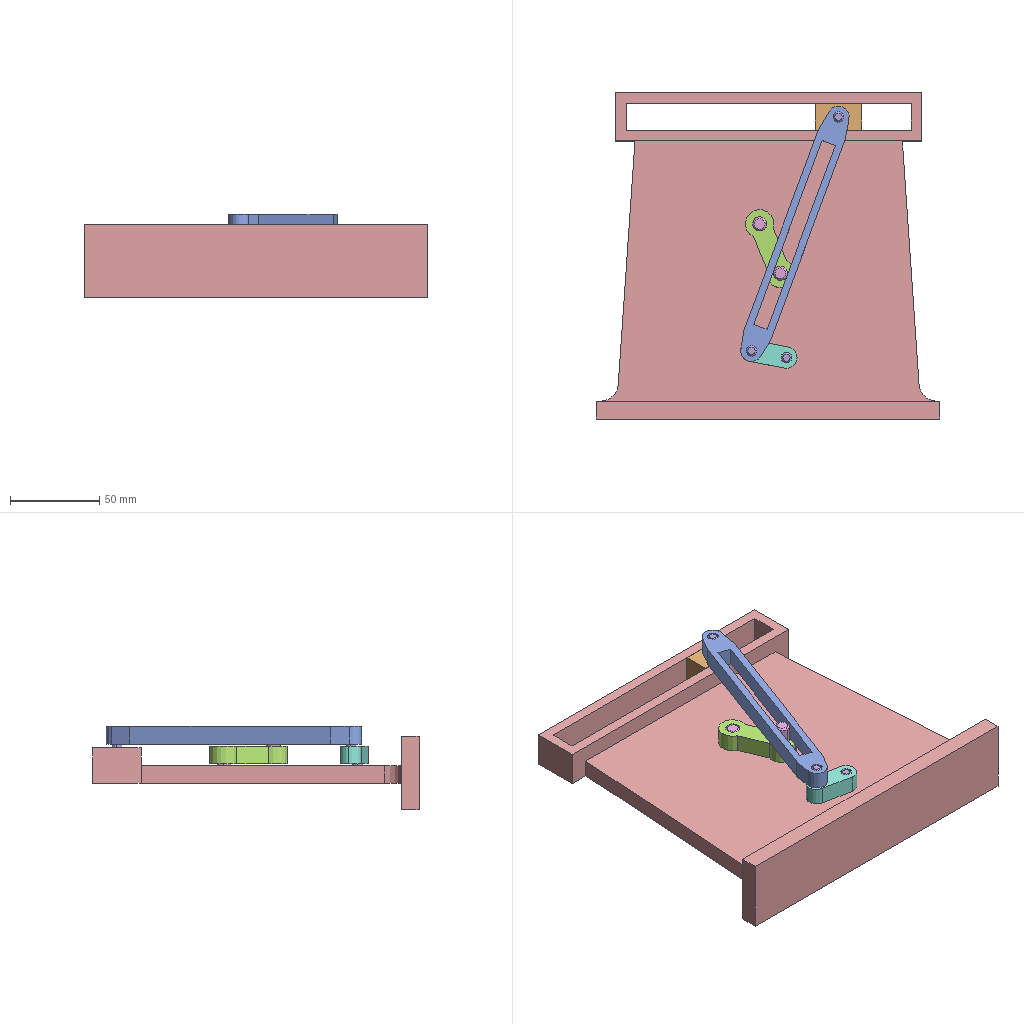Assembly | SolidWorks | 7 different items | 10 placed | box 193 x 183 x 47 mm
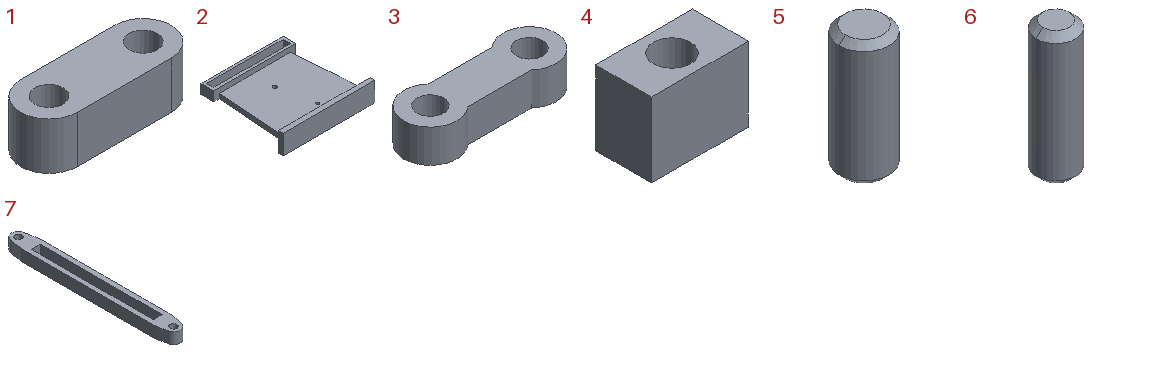Parts list (item | quantity | size | volume | features):
1 | x1 | 32 x 12 x 10 mm | 2965 mm3 | features Extrusion 1
2 | x1 | 192.506 x 183 x 41.072 mm | 357126 mm3 | features ICE 2, Extrusion 1, Fillet 1
3 | x1 | 46 x 16 x 10 mm | 4895 mm3 | features Extrusion 1
4 | x1 | 26 x 15 x 20 mm | 6229 mm3 | features Extrusion 1
5 | x2 | 8 x 8 x 20 mm | 982.271 mm3 | features Chamfer 1, Extrusion 1
6 | x3 | 6 x 6 x 20 mm | 548.732 mm3 | features Chamfer 1, Extrusion 1
7 | x1 | 16 x 152 x 10 mm | 13788 mm3 | features Extrusion 1
Mates (type | each side: item.copy, entity, surface, feature):
Concentric | 2.1 face cylinder Boss-Extrude1 | 3.1 face cylinder Boss-Extrude1
DistanceDim | 3.1 face plane Boss-Extrude1 | 2.1 face plane Boss-Extrude1
Concentric | 3.1 face cylinder Boss-Extrude1 | 5.1 face cylinder Boss-Extrude1
Coincident | 3.1 edge | 5.1 face plane Boss-Extrude1
DistanceDim | 7.1 face plane Boss-Extrude1 | 3.1 face plane Boss-Extrude1
Tangent | 7.1 face plane Boss-Extrude1 | 5.1 face cylinder Boss-Extrude1
Concentric | 2.1 face cylinder Boss-Extrude1 | 1.1 face cylinder Boss-Extrude1
Concentric | 7.1 face cylinder Boss-Extrude1 | 1.1 face cylinder Boss-Extrude1
Coincident | 2.1 face plane Boss-Extrude3 | 4.1 face plane Boss-Extrude1 | 2 times
Concentric | 7.1 face cylinder Boss-Extrude1 | 4.1 face cylinder Boss-Extrude1
Coincident | 3.1 face plane Boss-Extrude1 | 1.1 face plane Boss-Extrude1
Concentric | 3.1 face cylinder Boss-Extrude1 | 5.2 face cylinder Boss-Extrude1
Coincident | 3.1 face plane Boss-Extrude1 | 5.2 face plane Boss-Extrude1
Concentric | 7.1 face cylinder Boss-Extrude1 | 6.1 face cylinder Boss-Extrude1
Coincident | 7.1 face plane Boss-Extrude1 | 6.1 face plane Boss-Extrude1
Concentric | 7.1 face cylinder Boss-Extrude1 | 6.2 face cylinder Boss-Extrude1
Coincident | 7.1 face plane Boss-Extrude1 | 6.2 face plane Boss-Extrude1
Concentric | 1.1 face cylinder Boss-Extrude1 | 6.3 face cylinder Boss-Extrude1
Coincident | 1.1 face plane Boss-Extrude1 | 6.3 face plane Boss-Extrude1